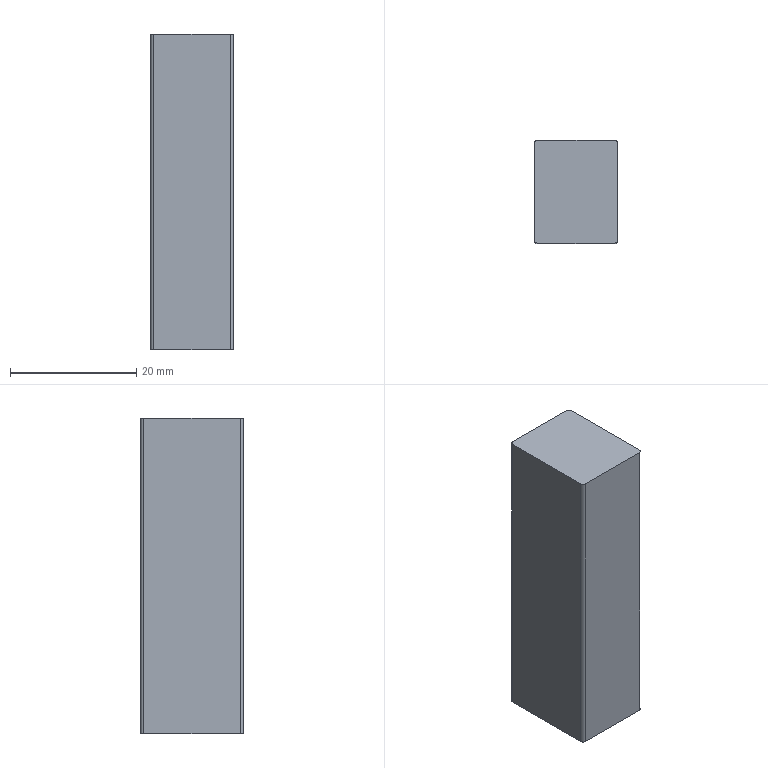Part | NX | features BREP 1 | 1 solid | 10 faces | box 13.115 x 16.326 x 50 mm | volume 10695 mm3 | plane 6 | cylinder 4 | commonest cylinder face diameters 1 x4
STEP:
#1=CARTESIAN_POINT('',(-6.058,8.163,-40.6));
#2=VERTEX_POINT('',#1);
#3=CARTESIAN_POINT('',(-6.558,7.663,-40.6));
#4=VERTEX_POINT('',#3);
#5=CARTESIAN_POINT('',(-6.058,7.663,-40.6));
#6=DIRECTION('',(0.,0.,1.));
#7=DIRECTION('',(1.,0.,0.));
#8=AXIS2_PLACEMENT_3D('',#5,#6,#7);
#9=CIRCLE('',#8,0.5);
#10=EDGE_CURVE('',#2,#4,#9,.T.);
#11=ORIENTED_EDGE('',*,*,#10,.F.);
#12=CARTESIAN_POINT('',(-6.058,8.163,-90.6));
#13=VERTEX_POINT('',#12);
#14=CARTESIAN_POINT('',(-6.058,8.163,-90.6));
#15=DIRECTION('',(0.,0.,1.));
#16=VECTOR('',#15,1000.);
#17=LINE('',#14,#16);
#18=EDGE_CURVE('',#13,#2,#17,.T.);
#19=ORIENTED_EDGE('',*,*,#18,.F.);
#20=CARTESIAN_POINT('',(-6.558,7.663,-90.6));
#21=VERTEX_POINT('',#20);
#22=CARTESIAN_POINT('',(-6.058,7.663,-90.6));
#23=DIRECTION('',(0.,0.,1.));
#24=DIRECTION('',(1.,0.,0.));
#25=AXIS2_PLACEMENT_3D('',#22,#23,#24);
#26=CIRCLE('',#25,0.5);
#27=EDGE_CURVE('',#13,#21,#26,.T.);
#28=ORIENTED_EDGE('',*,*,#27,.T.);
#29=CARTESIAN_POINT('',(-6.558,7.663,-90.6));
#30=DIRECTION('',(0.,0.,1.));
#31=VECTOR('',#30,1000.);
#32=LINE('',#29,#31);
#33=EDGE_CURVE('',#21,#4,#32,.T.);
#34=ORIENTED_EDGE('',*,*,#33,.T.);
#35=EDGE_LOOP('',(#11,#19,#28,#34));
#36=FACE_BOUND('',#35,.T.);
#37=CARTESIAN_POINT('',(-6.058,7.663,-90.6));
#38=DIRECTION('',(0.,0.,1.));
#39=DIRECTION('',(-1.,0.,0.));
#40=AXIS2_PLACEMENT_3D('',#37,#38,#39);
#41=CYLINDRICAL_SURFACE('',#40,0.5);
#42=ADVANCED_FACE('',(#36),#41,.T.);
#43=CARTESIAN_POINT('',(-6.558,-7.663,-40.6));
#44=VERTEX_POINT('',#43);
#45=CARTESIAN_POINT('',(-6.558,-7.663,-40.6));
#46=DIRECTION('',(0.,1.,0.));
#47=VECTOR('',#46,1000.);
#48=LINE('',#45,#47);
#49=EDGE_CURVE('',#44,#4,#48,.T.);
#50=ORIENTED_EDGE('',*,*,#49,.T.);
#51=ORIENTED_EDGE('',*,*,#33,.F.);
#52=CARTESIAN_POINT('',(-6.558,-7.663,-90.6));
#53=VERTEX_POINT('',#52);
#54=CARTESIAN_POINT('',(-6.558,-7.663,-90.6));
#55=DIRECTION('',(0.,1.,0.));
#56=VECTOR('',#55,1000.);
#57=LINE('',#54,#56);
#58=EDGE_CURVE('',#53,#21,#57,.T.);
#59=ORIENTED_EDGE('',*,*,#58,.F.);
#60=CARTESIAN_POINT('',(-6.558,-7.663,-90.6));
#61=DIRECTION('',(0.,0.,1.));
#62=VECTOR('',#61,1000.);
#63=LINE('',#60,#62);
#64=EDGE_CURVE('',#53,#44,#63,.T.);
#65=ORIENTED_EDGE('',*,*,#64,.T.);
#66=EDGE_LOOP('',(#50,#51,#59,#65));
#67=FACE_BOUND('',#66,.T.);
#68=CARTESIAN_POINT('',(-6.558,-7.663,-90.6));
#69=DIRECTION('',(1.,0.,0.));
#70=DIRECTION('',(0.,0.,1.));
#71=AXIS2_PLACEMENT_3D('',#68,#69,#70);
#72=PLANE('',#71);
#73=ADVANCED_FACE('',(#67),#72,.F.);
#74=CARTESIAN_POINT('',(-6.058,-8.163,-40.6));
#75=VERTEX_POINT('',#74);
#76=CARTESIAN_POINT('',(-6.058,-7.663,-40.6));
#77=DIRECTION('',(0.,0.,1.));
#78=DIRECTION('',(1.,0.,0.));
#79=AXIS2_PLACEMENT_3D('',#76,#77,#78);
#80=CIRCLE('',#79,0.5);
#81=EDGE_CURVE('',#44,#75,#80,.T.);
#82=ORIENTED_EDGE('',*,*,#81,.F.);
#83=ORIENTED_EDGE('',*,*,#64,.F.);
#84=CARTESIAN_POINT('',(-6.058,-8.163,-90.6));
#85=VERTEX_POINT('',#84);
#86=CARTESIAN_POINT('',(-6.058,-7.663,-90.6));
#87=DIRECTION('',(0.,0.,1.));
#88=DIRECTION('',(1.,0.,0.));
#89=AXIS2_PLACEMENT_3D('',#86,#87,#88);
#90=CIRCLE('',#89,0.5);
#91=EDGE_CURVE('',#53,#85,#90,.T.);
#92=ORIENTED_EDGE('',*,*,#91,.T.);
#93=CARTESIAN_POINT('',(-6.058,-8.163,-90.6));
#94=DIRECTION('',(0.,0.,1.));
#95=VECTOR('',#94,1000.);
#96=LINE('',#93,#95);
#97=EDGE_CURVE('',#85,#75,#96,.T.);
#98=ORIENTED_EDGE('',*,*,#97,.T.);
#99=EDGE_LOOP('',(#82,#83,#92,#98));
#100=FACE_BOUND('',#99,.T.);
#101=CARTESIAN_POINT('',(-6.058,-7.663,-90.6));
#102=DIRECTION('',(0.,0.,1.));
#103=DIRECTION('',(-1.,0.,0.));
#104=AXIS2_PLACEMENT_3D('',#101,#102,#103);
#105=CYLINDRICAL_SURFACE('',#104,0.5);
#106=ADVANCED_FACE('',(#100),#105,.T.);
#107=CARTESIAN_POINT('',(6.058,-8.163,-40.6));
#108=VERTEX_POINT('',#107);
#109=CARTESIAN_POINT('',(6.058,-8.163,-40.6));
#110=DIRECTION('',(-1.,0.,0.));
#111=VECTOR('',#110,1000.);
#112=LINE('',#109,#111);
#113=EDGE_CURVE('',#108,#75,#112,.T.);
#114=ORIENTED_EDGE('',*,*,#113,.T.);
#115=ORIENTED_EDGE('',*,*,#97,.F.);
#116=CARTESIAN_POINT('',(6.058,-8.163,-90.6));
#117=VERTEX_POINT('',#116);
#118=CARTESIAN_POINT('',(6.058,-8.163,-90.6));
#119=DIRECTION('',(-1.,0.,0.));
#120=VECTOR('',#119,1000.);
#121=LINE('',#118,#120);
#122=EDGE_CURVE('',#117,#85,#121,.T.);
#123=ORIENTED_EDGE('',*,*,#122,.F.);
#124=CARTESIAN_POINT('',(6.058,-8.163,-90.6));
#125=DIRECTION('',(0.,0.,1.));
#126=VECTOR('',#125,1000.);
#127=LINE('',#124,#126);
#128=EDGE_CURVE('',#117,#108,#127,.T.);
#129=ORIENTED_EDGE('',*,*,#128,.T.);
#130=EDGE_LOOP('',(#114,#115,#123,#129));
#131=FACE_BOUND('',#130,.T.);
#132=CARTESIAN_POINT('',(6.058,-8.163,-90.6));
#133=DIRECTION('',(0.,1.,0.));
#134=DIRECTION('',(0.,0.,-1.));
#135=AXIS2_PLACEMENT_3D('',#132,#133,#134);
#136=PLANE('',#135);
#137=ADVANCED_FACE('',(#131),#136,.F.);
#138=CARTESIAN_POINT('',(6.558,-7.663,-40.6));
#139=VERTEX_POINT('',#138);
#140=CARTESIAN_POINT('',(6.058,-7.663,-40.6));
#141=DIRECTION('',(0.,0.,1.));
#142=DIRECTION('',(1.,0.,0.));
#143=AXIS2_PLACEMENT_3D('',#140,#141,#142);
#144=CIRCLE('',#143,0.5);
#145=EDGE_CURVE('',#108,#139,#144,.T.);
#146=ORIENTED_EDGE('',*,*,#145,.F.);
#147=ORIENTED_EDGE('',*,*,#128,.F.);
#148=CARTESIAN_POINT('',(6.558,-7.663,-90.6));
#149=VERTEX_POINT('',#148);
#150=CARTESIAN_POINT('',(6.058,-7.663,-90.6));
#151=DIRECTION('',(0.,0.,1.));
#152=DIRECTION('',(1.,0.,0.));
#153=AXIS2_PLACEMENT_3D('',#150,#151,#152);
#154=CIRCLE('',#153,0.5);
#155=EDGE_CURVE('',#117,#149,#154,.T.);
#156=ORIENTED_EDGE('',*,*,#155,.T.);
#157=CARTESIAN_POINT('',(6.558,-7.663,-90.6));
#158=DIRECTION('',(0.,0.,1.));
#159=VECTOR('',#158,1000.);
#160=LINE('',#157,#159);
#161=EDGE_CURVE('',#149,#139,#160,.T.);
#162=ORIENTED_EDGE('',*,*,#161,.T.);
#163=EDGE_LOOP('',(#146,#147,#156,#162));
#164=FACE_BOUND('',#163,.T.);
#165=CARTESIAN_POINT('',(6.058,-7.663,-90.6));
#166=DIRECTION('',(0.,0.,1.));
#167=DIRECTION('',(-1.,0.,0.));
#168=AXIS2_PLACEMENT_3D('',#165,#166,#167);
#169=CYLINDRICAL_SURFACE('',#168,0.5);
#170=ADVANCED_FACE('',(#164),#169,.T.);
#171=CARTESIAN_POINT('',(6.558,7.663,-40.6));
#172=VERTEX_POINT('',#171);
#173=CARTESIAN_POINT('',(6.558,7.663,-40.6));
#174=DIRECTION('',(0.,-1.,0.));
#175=VECTOR('',#174,1000.);
#176=LINE('',#173,#175);
#177=EDGE_CURVE('',#172,#139,#176,.T.);
#178=ORIENTED_EDGE('',*,*,#177,.T.);
#179=ORIENTED_EDGE('',*,*,#161,.F.);
#180=CARTESIAN_POINT('',(6.558,7.663,-90.6));
#181=VERTEX_POINT('',#180);
#182=CARTESIAN_POINT('',(6.558,7.663,-90.6));
#183=DIRECTION('',(0.,-1.,0.));
#184=VECTOR('',#183,1000.);
#185=LINE('',#182,#184);
#186=EDGE_CURVE('',#181,#149,#185,.T.);
#187=ORIENTED_EDGE('',*,*,#186,.F.);
#188=CARTESIAN_POINT('',(6.558,7.663,-90.6));
#189=DIRECTION('',(0.,0.,1.));
#190=VECTOR('',#189,1000.);
#191=LINE('',#188,#190);
#192=EDGE_CURVE('',#181,#172,#191,.T.);
#193=ORIENTED_EDGE('',*,*,#192,.T.);
#194=EDGE_LOOP('',(#178,#179,#187,#193));
#195=FACE_BOUND('',#194,.T.);
#196=CARTESIAN_POINT('',(6.558,7.663,-90.6));
#197=DIRECTION('',(-1.,0.,0.));
#198=DIRECTION('',(0.,1.,0.));
#199=AXIS2_PLACEMENT_3D('',#196,#197,#198);
#200=PLANE('',#199);
#201=ADVANCED_FACE('',(#195),#200,.F.);
#202=CARTESIAN_POINT('',(6.058,8.163,-40.6));
#203=VERTEX_POINT('',#202);
#204=CARTESIAN_POINT('',(6.058,7.663,-40.6));
#205=DIRECTION('',(0.,0.,1.));
#206=DIRECTION('',(1.,0.,0.));
#207=AXIS2_PLACEMENT_3D('',#204,#205,#206);
#208=CIRCLE('',#207,0.5);
#209=EDGE_CURVE('',#172,#203,#208,.T.);
#210=ORIENTED_EDGE('',*,*,#209,.F.);
#211=ORIENTED_EDGE('',*,*,#192,.F.);
#212=CARTESIAN_POINT('',(6.058,8.163,-90.6));
#213=VERTEX_POINT('',#212);
#214=CARTESIAN_POINT('',(6.058,7.663,-90.6));
#215=DIRECTION('',(0.,0.,1.));
#216=DIRECTION('',(1.,0.,0.));
#217=AXIS2_PLACEMENT_3D('',#214,#215,#216);
#218=CIRCLE('',#217,0.5);
#219=EDGE_CURVE('',#181,#213,#218,.T.);
#220=ORIENTED_EDGE('',*,*,#219,.T.);
#221=CARTESIAN_POINT('',(6.058,8.163,-90.6));
#222=DIRECTION('',(0.,0.,1.));
#223=VECTOR('',#222,1000.);
#224=LINE('',#221,#223);
#225=EDGE_CURVE('',#213,#203,#224,.T.);
#226=ORIENTED_EDGE('',*,*,#225,.T.);
#227=EDGE_LOOP('',(#210,#211,#220,#226));
#228=FACE_BOUND('',#227,.T.);
#229=CARTESIAN_POINT('',(6.058,7.663,-90.6));
#230=DIRECTION('',(0.,0.,1.));
#231=DIRECTION('',(-1.,0.,0.));
#232=AXIS2_PLACEMENT_3D('',#229,#230,#231);
#233=CYLINDRICAL_SURFACE('',#232,0.5);
#234=ADVANCED_FACE('',(#228),#233,.T.);
#235=CARTESIAN_POINT('',(-6.058,8.163,-40.6));
#236=DIRECTION('',(1.,0.,0.));
#237=VECTOR('',#236,1000.);
#238=LINE('',#235,#237);
#239=EDGE_CURVE('',#2,#203,#238,.T.);
#240=ORIENTED_EDGE('',*,*,#239,.T.);
#241=ORIENTED_EDGE('',*,*,#225,.F.);
#242=CARTESIAN_POINT('',(-6.058,8.163,-90.6));
#243=DIRECTION('',(1.,0.,0.));
#244=VECTOR('',#243,1000.);
#245=LINE('',#242,#244);
#246=EDGE_CURVE('',#13,#213,#245,.T.);
#247=ORIENTED_EDGE('',*,*,#246,.F.);
#248=ORIENTED_EDGE('',*,*,#18,.T.);
#249=EDGE_LOOP('',(#240,#241,#247,#248));
#250=FACE_BOUND('',#249,.T.);
#251=CARTESIAN_POINT('',(-6.058,8.163,-90.6));
#252=DIRECTION('',(0.,-1.,0.));
#253=DIRECTION('',(-1.,0.,0.));
#254=AXIS2_PLACEMENT_3D('',#251,#252,#253);
#255=PLANE('',#254);
#256=ADVANCED_FACE('',(#250),#255,.F.);
#257=ORIENTED_EDGE('',*,*,#27,.F.);
#258=ORIENTED_EDGE('',*,*,#246,.T.);
#259=ORIENTED_EDGE('',*,*,#219,.F.);
#260=ORIENTED_EDGE('',*,*,#186,.T.);
#261=ORIENTED_EDGE('',*,*,#155,.F.);
#262=ORIENTED_EDGE('',*,*,#122,.T.);
#263=ORIENTED_EDGE('',*,*,#91,.F.);
#264=ORIENTED_EDGE('',*,*,#58,.T.);
#265=EDGE_LOOP('',(#257,#258,#259,#260,#261,#262,#263,#264));
#266=FACE_BOUND('',#265,.T.);
#267=CARTESIAN_POINT('',(-6.058,7.663,-90.6));
#268=DIRECTION('',(0.,0.,1.));
#269=DIRECTION('',(-1.,0.,0.));
#270=AXIS2_PLACEMENT_3D('',#267,#268,#269);
#271=PLANE('',#270);
#272=ADVANCED_FACE('',(#266),#271,.F.);
#273=ORIENTED_EDGE('',*,*,#10,.T.);
#274=ORIENTED_EDGE('',*,*,#49,.F.);
#275=ORIENTED_EDGE('',*,*,#81,.T.);
#276=ORIENTED_EDGE('',*,*,#113,.F.);
#277=ORIENTED_EDGE('',*,*,#145,.T.);
#278=ORIENTED_EDGE('',*,*,#177,.F.);
#279=ORIENTED_EDGE('',*,*,#209,.T.);
#280=ORIENTED_EDGE('',*,*,#239,.F.);
#281=EDGE_LOOP('',(#273,#274,#275,#276,#277,#278,#279,#280));
#282=FACE_BOUND('',#281,.T.);
#283=CARTESIAN_POINT('',(-6.058,7.663,-40.6));
#284=DIRECTION('',(0.,0.,1.));
#285=DIRECTION('',(-1.,0.,0.));
#286=AXIS2_PLACEMENT_3D('',#283,#284,#285);
#287=PLANE('',#286);
#288=ADVANCED_FACE('',(#282),#287,.T.);
#289=CLOSED_SHELL('',(#42,#73,#106,#137,#170,#201,#234,#256,#272,#288));
#290=MANIFOLD_SOLID_BREP('',#289);
#291=(LENGTH_UNIT()NAMED_UNIT(*)SI_UNIT(.MILLI.,.METRE.));
#292=UNCERTAINTY_MEASURE_WITH_UNIT(LENGTH_MEASURE(0.00001),#291,'','');
#293=(NAMED_UNIT(*)PLANE_ANGLE_UNIT()SI_UNIT($,.RADIAN.));
#294=(NAMED_UNIT(*)SI_UNIT($,.STERADIAN.)SOLID_ANGLE_UNIT());
#295=(GEOMETRIC_REPRESENTATION_CONTEXT(3)GLOBAL_UNCERTAINTY_ASSIGNED_CONTEXT((#292))GLOBAL_UNIT_ASSIGNED_CONTEXT((#291,#293,#294))REPRESENTATION_CONTEXT('',''));
#296=ADVANCED_BREP_SHAPE_REPRESENTATION('',(#290),#295);